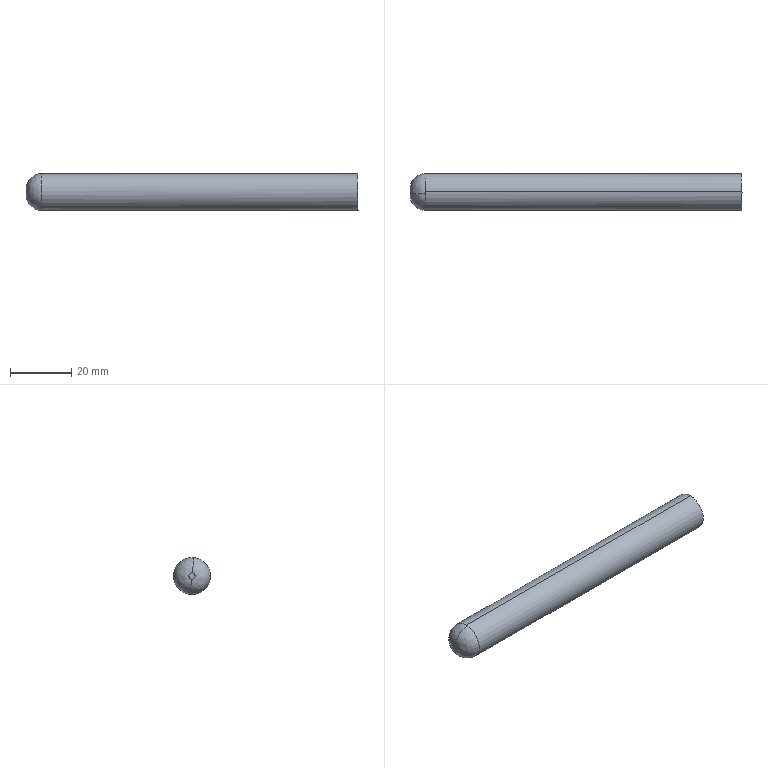Part | Creo | 1 solid | 6 faces | box 108.147 x 12 x 12 mm | volume 12066 mm3 | plane 2 | cylinder 2 | spline 2 | commonest cylinder face diameters 12 x2
STEP:
#1=CARTESIAN_POINT('',(0.,0.,0.));
#2=DIRECTION('',(0.,0.,1.));
#3=DIRECTION('',(1.,0.,0.));
#4=AXIS2_PLACEMENT_3D('',#1,#2,#3);
#5=CARTESIAN_POINT('',(-42.553,96.983,-27.835));
#6=VERTEX_POINT('',#5);
#7=CARTESIAN_POINT('',(-42.553,96.353,-39.802));
#8=VERTEX_POINT('',#7);
#9=CARTESIAN_POINT('',(-42.553,96.983,-33.835));
#10=DIRECTION('',(1.,0.,0.000000164));
#11=DIRECTION('',(-0.000000164,-0.00000002,1.));
#12=AXIS2_PLACEMENT_3D('',#9,#10,#11);
#13=CIRCLE('',#12,6.);
#14=EDGE_CURVE('',#6,#8,#13,.T.);
#15=ORIENTED_EDGE('',*,*,#14,.F.);
#16=CARTESIAN_POINT('',(-42.553,96.983,-39.835));
#17=VERTEX_POINT('',#16);
#18=CARTESIAN_POINT('',(-42.553,96.983,-33.835));
#19=DIRECTION('',(1.,0.,0.000000164));
#20=DIRECTION('',(0.000000164,0.,-1.));
#21=AXIS2_PLACEMENT_3D('',#18,#19,#20);
#22=CIRCLE('',#21,6.);
#23=EDGE_CURVE('',#17,#6,#22,.T.);
#24=ORIENTED_EDGE('',*,*,#23,.F.);
#25=CARTESIAN_POINT('',(-42.553,96.983,-33.835));
#26=DIRECTION('',(1.,0.,0.000000164));
#27=DIRECTION('',(0.000000164,-0.1051,-0.9945));
#28=AXIS2_PLACEMENT_3D('',#25,#26,#27);
#29=CIRCLE('',#28,6.);
#30=EDGE_CURVE('',#8,#17,#29,.T.);
#31=ORIENTED_EDGE('',*,*,#30,.F.);
#32=EDGE_LOOP('',(#15,#24,#31));
#33=FACE_OUTER_BOUND('',#32,.F.);
#34=CARTESIAN_POINT('',(-42.553,96.983,-33.835));
#35=DIRECTION('',(1.,0.,0.000000197));
#36=DIRECTION('',(0.000000197,0.,-1.));
#37=AXIS2_PLACEMENT_3D('',#34,#35,#36);
#38=PLANE('',#37);
#39=ADVANCED_FACE('',(#33),#38,.T.);
#40=CARTESIAN_POINT('',(-145.7,96.983,-39.835));
#41=VERTEX_POINT('',#40);
#42=CARTESIAN_POINT('',(-145.7,96.353,-27.869));
#43=VERTEX_POINT('',#42);
#44=CARTESIAN_POINT('',(-145.7,96.983,-33.835));
#45=DIRECTION('',(-1.,0.,-0.000000164));
#46=DIRECTION('',(0.000000164,0.,-1.));
#47=AXIS2_PLACEMENT_3D('',#44,#45,#46);
#48=CIRCLE('',#47,6.);
#49=EDGE_CURVE('',#41,#43,#48,.T.);
#50=ORIENTED_EDGE('',*,*,#49,.T.);
#51=CARTESIAN_POINT('',(-145.7,96.983,-27.835));
#52=VERTEX_POINT('',#51);
#53=CARTESIAN_POINT('',(-145.7,96.983,-33.835));
#54=DIRECTION('',(-1.,0.,-0.000000164));
#55=DIRECTION('',(-0.000000164,-0.1051,0.9945));
#56=AXIS2_PLACEMENT_3D('',#53,#54,#55);
#57=CIRCLE('',#56,6.);
#58=EDGE_CURVE('',#43,#52,#57,.T.);
#59=ORIENTED_EDGE('',*,*,#58,.T.);
#60=CARTESIAN_POINT('',(-42.553,96.983,-27.835));
#61=DIRECTION('',(-1.,-0.00000186,0.000000408));
#62=VECTOR('',#61,103.147);
#63=LINE('',#60,#62);
#64=EDGE_CURVE('',#6,#52,#63,.T.);
#65=ORIENTED_EDGE('',*,*,#64,.F.);
#66=ORIENTED_EDGE('',*,*,#14,.T.);
#67=ORIENTED_EDGE('',*,*,#30,.T.);
#68=CARTESIAN_POINT('',(-42.553,96.983,-39.835));
#69=DIRECTION('',(-1.,0.000001529,-0.000000164));
#70=VECTOR('',#69,103.147);
#71=LINE('',#68,#70);
#72=EDGE_CURVE('',#17,#41,#71,.T.);
#73=ORIENTED_EDGE('',*,*,#72,.T.);
#74=EDGE_LOOP('',(#50,#59,#65,#66,#67,#73));
#75=FACE_OUTER_BOUND('',#74,.F.);
#76=CARTESIAN_POINT('',(-121.87,96.983,-33.835));
#77=DIRECTION('',(-1.,0.,-0.000000164));
#78=DIRECTION('',(-0.000000164,0.,1.));
#79=AXIS2_PLACEMENT_3D('',#76,#77,#78);
#80=CYLINDRICAL_SURFACE('',#79,6.);
#81=ADVANCED_FACE('',(#75),#80,.T.);
#82=CARTESIAN_POINT('',(-145.7,97.613,-39.802));
#83=VERTEX_POINT('',#82);
#84=CARTESIAN_POINT('',(-145.7,96.983,-33.835));
#85=DIRECTION('',(-1.,0.,-0.000000164));
#86=DIRECTION('',(0.000000164,0.1051,-0.9945));
#87=AXIS2_PLACEMENT_3D('',#84,#85,#86);
#88=CIRCLE('',#87,6.);
#89=EDGE_CURVE('',#83,#41,#88,.T.);
#90=ORIENTED_EDGE('',*,*,#89,.F.);
#91=CARTESIAN_POINT('',(-150.7,97.088,-34.83));
#92=VERTEX_POINT('',#91);
#93=CARTESIAN_POINT('',(-145.7,97.088,-34.83));
#94=DIRECTION('',(0.000000017,-0.9945,-0.1051));
#95=DIRECTION('',(-1.,0.,-0.000000164));
#96=AXIS2_PLACEMENT_3D('',#93,#94,#95);
#97=CIRCLE('',#96,5.);
#98=EDGE_CURVE('',#92,#83,#97,.T.);
#99=ORIENTED_EDGE('',*,*,#98,.F.);
#100=CARTESIAN_POINT('',(-150.7,96.878,-32.841));
#101=VERTEX_POINT('',#100);
#102=CARTESIAN_POINT('',(-150.7,96.878,-32.841));
#103=CARTESIAN_POINT('',(-150.7,96.772,-32.852));
#104=CARTESIAN_POINT('',(-150.7,96.574,-32.905));
#105=CARTESIAN_POINT('',(-150.7,96.302,-33.079));
#106=CARTESIAN_POINT('',(-150.7,96.1,-33.331));
#107=CARTESIAN_POINT('',(-150.7,95.987,-33.63));
#108=CARTESIAN_POINT('',(-150.7,95.973,-33.948));
#109=CARTESIAN_POINT('',(-150.7,96.056,-34.252));
#110=CARTESIAN_POINT('',(-150.7,96.228,-34.516));
#111=CARTESIAN_POINT('',(-150.7,96.474,-34.716));
#112=CARTESIAN_POINT('',(-150.7,96.777,-34.83));
#113=CARTESIAN_POINT('',(-150.7,96.982,-34.841));
#114=CARTESIAN_POINT('',(-150.7,97.088,-34.83));
#115=B_SPLINE_CURVE_WITH_KNOTS('',3,(#102,#103,#104,#105,#106,#107,#108,#109,#110,#111,#112,#113,#114),.UNSPECIFIED.,.F.,.F.,(4,1,1,1,1,1,1,1,1,1,4),(0.,0.1,0.2,0.3,0.4,0.5,0.6,0.7,0.8,0.9,1.),.UNSPECIFIED.);
#116=EDGE_CURVE('',#101,#92,#115,.T.);
#117=ORIENTED_EDGE('',*,*,#116,.F.);
#118=CARTESIAN_POINT('',(-145.7,96.878,-32.841));
#119=DIRECTION('',(-0.000000017,0.9945,0.1051));
#120=DIRECTION('',(-1.,0.000000835,-0.00000807));
#121=AXIS2_PLACEMENT_3D('',#118,#119,#120);
#122=CIRCLE('',#121,5.);
#123=EDGE_CURVE('',#101,#43,#122,.T.);
#124=ORIENTED_EDGE('',*,*,#123,.T.);
#125=ORIENTED_EDGE('',*,*,#49,.F.);
#126=EDGE_LOOP('',(#90,#99,#117,#124,#125));
#127=FACE_OUTER_BOUND('',#126,.F.);
#128=CARTESIAN_POINT('',(-150.697,97.005,-32.994));
#129=CARTESIAN_POINT('',(-150.795,97.086,-29.919));
#130=CARTESIAN_POINT('',(-148.619,97.143,-27.743));
#131=CARTESIAN_POINT('',(-145.543,97.14,-27.84));
#132=CARTESIAN_POINT('',(-150.697,96.459,-32.979));
#133=CARTESIAN_POINT('',(-150.795,94.545,-29.852));
#134=CARTESIAN_POINT('',(-148.619,93.19,-27.639));
#135=CARTESIAN_POINT('',(-145.543,93.25,-27.738));
#136=CARTESIAN_POINT('',(-150.697,96.088,-33.381));
#137=CARTESIAN_POINT('',(-150.795,92.82,-31.719));
#138=CARTESIAN_POINT('',(-148.619,90.507,-30.544));
#139=CARTESIAN_POINT('',(-145.543,90.61,-30.596));
#140=CARTESIAN_POINT('',(-150.697,96.146,-33.924));
#141=CARTESIAN_POINT('',(-150.795,93.087,-34.247));
#142=CARTESIAN_POINT('',(-148.619,90.923,-34.476));
#143=CARTESIAN_POINT('',(-145.543,91.019,-34.466));
#144=CARTESIAN_POINT('',(-150.697,96.203,-34.467));
#145=CARTESIAN_POINT('',(-150.795,93.354,-36.775));
#146=CARTESIAN_POINT('',(-148.619,91.338,-38.408));
#147=CARTESIAN_POINT('',(-145.543,91.428,-38.335));
#148=CARTESIAN_POINT('',(-150.697,96.65,-34.782));
#149=CARTESIAN_POINT('',(-150.795,95.431,-38.24));
#150=CARTESIAN_POINT('',(-148.619,94.569,-40.687));
#151=CARTESIAN_POINT('',(-145.543,94.607,-40.578));
#152=CARTESIAN_POINT('',(-150.697,97.18,-34.654));
#153=CARTESIAN_POINT('',(-150.795,97.902,-37.644));
#154=CARTESIAN_POINT('',(-148.619,98.413,-39.76));
#155=CARTESIAN_POINT('',(-145.543,98.39,-39.666));
#156=(BOUNDED_SURFACE()B_SPLINE_SURFACE(3,3,((#128,#129,#130,#131),(#132,#133,#134,#135),(#136,#137,#138,#139),(#140,#141,#142,#143),(#144,#145,#146,#147),(#148,#149,#150,#151),(#152,#153,#154,#155)),.UNSPECIFIED.,.F.,.F.,.F.)B_SPLINE_SURFACE_WITH_KNOTS((4,3,4),(4,4),(0.,1.,2.),(0.,1.),.UNSPECIFIED.)GEOMETRIC_REPRESENTATION_ITEM()RATIONAL_B_SPLINE_SURFACE(((1.431,1.13,1.13,1.431),(1.106,0.8733,0.8733,1.106),(1.106,0.8733,0.8733,1.106),(1.431,1.13,1.13,1.431),(1.106,0.8733,0.8733,1.106),(1.106,0.8733,0.8733,1.106),(1.431,1.13,1.13,1.431)))REPRESENTATION_ITEM('')SURFACE());
#157=ADVANCED_FACE('',(#127),#156,.T.);
#158=ORIENTED_EDGE('',*,*,#89,.T.);
#159=ORIENTED_EDGE('',*,*,#72,.F.);
#160=ORIENTED_EDGE('',*,*,#23,.T.);
#161=ORIENTED_EDGE('',*,*,#64,.T.);
#162=CARTESIAN_POINT('',(-145.7,96.983,-33.835));
#163=DIRECTION('',(-1.,0.,-0.000000164));
#164=DIRECTION('',(-0.000000164,0.,1.));
#165=AXIS2_PLACEMENT_3D('',#162,#163,#164);
#166=CIRCLE('',#165,6.);
#167=EDGE_CURVE('',#52,#83,#166,.T.);
#168=ORIENTED_EDGE('',*,*,#167,.T.);
#169=EDGE_LOOP('',(#158,#159,#160,#161,#168));
#170=FACE_OUTER_BOUND('',#169,.F.);
#171=CARTESIAN_POINT('',(-121.87,96.983,-33.835));
#172=DIRECTION('',(-1.,0.,-0.000000164));
#173=DIRECTION('',(-0.000000164,0.,1.));
#174=AXIS2_PLACEMENT_3D('',#171,#172,#173);
#175=CYLINDRICAL_SURFACE('',#174,6.);
#176=ADVANCED_FACE('',(#170),#175,.T.);
#177=ORIENTED_EDGE('',*,*,#58,.F.);
#178=ORIENTED_EDGE('',*,*,#123,.F.);
#179=CARTESIAN_POINT('',(-150.7,97.088,-34.83));
#180=CARTESIAN_POINT('',(-150.7,97.194,-34.819));
#181=CARTESIAN_POINT('',(-150.7,97.393,-34.765));
#182=CARTESIAN_POINT('',(-150.7,97.664,-34.591));
#183=CARTESIAN_POINT('',(-150.7,97.866,-34.34));
#184=CARTESIAN_POINT('',(-150.7,97.979,-34.04));
#185=CARTESIAN_POINT('',(-150.7,97.993,-33.722));
#186=CARTESIAN_POINT('',(-150.7,97.909,-33.418));
#187=CARTESIAN_POINT('',(-150.7,97.739,-33.156));
#188=CARTESIAN_POINT('',(-150.7,97.493,-32.955));
#189=CARTESIAN_POINT('',(-150.7,97.188,-32.84));
#190=CARTESIAN_POINT('',(-150.7,96.984,-32.83));
#191=CARTESIAN_POINT('',(-150.7,96.878,-32.841));
#192=B_SPLINE_CURVE_WITH_KNOTS('',3,(#179,#180,#181,#182,#183,#184,#185,#186,#187,#188,#189,#190,#191),.UNSPECIFIED.,.F.,.F.,(4,1,1,1,1,1,1,1,1,1,4),(0.,0.1,0.2,0.3,0.4,0.5,0.6,0.7,0.8,0.9,1.),.UNSPECIFIED.);
#193=EDGE_CURVE('',#92,#101,#192,.T.);
#194=ORIENTED_EDGE('',*,*,#193,.F.);
#195=ORIENTED_EDGE('',*,*,#98,.T.);
#196=ORIENTED_EDGE('',*,*,#167,.F.);
#197=EDGE_LOOP('',(#177,#178,#194,#195,#196));
#198=FACE_OUTER_BOUND('',#197,.F.);
#199=CARTESIAN_POINT('',(-150.697,96.961,-34.677));
#200=CARTESIAN_POINT('',(-150.795,96.88,-37.752));
#201=CARTESIAN_POINT('',(-148.619,96.823,-39.927));
#202=CARTESIAN_POINT('',(-145.543,96.826,-39.831));
#203=CARTESIAN_POINT('',(-150.697,97.507,-34.691));
#204=CARTESIAN_POINT('',(-150.795,99.421,-37.819));
#205=CARTESIAN_POINT('',(-148.619,100.776,-40.031));
#206=CARTESIAN_POINT('',(-145.543,100.716,-39.933));
#207=CARTESIAN_POINT('',(-150.697,97.878,-34.29));
#208=CARTESIAN_POINT('',(-150.795,101.146,-35.952));
#209=CARTESIAN_POINT('',(-148.619,103.459,-37.127));
#210=CARTESIAN_POINT('',(-145.543,103.356,-37.075));
#211=CARTESIAN_POINT('',(-150.697,97.82,-33.747));
#212=CARTESIAN_POINT('',(-150.795,100.879,-33.424));
#213=CARTESIAN_POINT('',(-148.619,103.043,-33.195));
#214=CARTESIAN_POINT('',(-145.543,102.947,-33.205));
#215=CARTESIAN_POINT('',(-150.697,97.763,-33.204));
#216=CARTESIAN_POINT('',(-150.795,100.612,-30.896));
#217=CARTESIAN_POINT('',(-148.619,102.628,-29.263));
#218=CARTESIAN_POINT('',(-145.543,102.538,-29.335));
#219=CARTESIAN_POINT('',(-150.697,97.316,-32.889));
#220=CARTESIAN_POINT('',(-150.795,98.535,-29.431));
#221=CARTESIAN_POINT('',(-148.619,99.397,-26.984));
#222=CARTESIAN_POINT('',(-145.543,99.359,-27.092));
#223=CARTESIAN_POINT('',(-150.697,96.786,-33.017));
#224=CARTESIAN_POINT('',(-150.795,96.064,-30.027));
#225=CARTESIAN_POINT('',(-148.619,95.553,-27.911));
#226=CARTESIAN_POINT('',(-145.543,95.576,-28.005));
#227=(BOUNDED_SURFACE()B_SPLINE_SURFACE(3,3,((#199,#200,#201,#202),(#203,#204,#205,#206),(#207,#208,#209,#210),(#211,#212,#213,#214),(#215,#216,#217,#218),(#219,#220,#221,#222),(#223,#224,#225,#226)),.UNSPECIFIED.,.F.,.F.,.F.)B_SPLINE_SURFACE_WITH_KNOTS((4,3,4),(4,4),(0.,1.,2.),(0.,1.),.UNSPECIFIED.)GEOMETRIC_REPRESENTATION_ITEM()RATIONAL_B_SPLINE_SURFACE(((1.431,1.13,1.13,1.431),(1.106,0.8733,0.8733,1.106),(1.106,0.8733,0.8733,1.106),(1.431,1.13,1.13,1.431),(1.106,0.8733,0.8733,1.106),(1.106,0.8733,0.8733,1.106),(1.431,1.13,1.13,1.431)))REPRESENTATION_ITEM('')SURFACE());
#228=ADVANCED_FACE('',(#198),#227,.T.);
#229=ORIENTED_EDGE('',*,*,#193,.T.);
#230=ORIENTED_EDGE('',*,*,#116,.T.);
#231=EDGE_LOOP('',(#229,#230));
#232=FACE_OUTER_BOUND('',#231,.F.);
#233=CARTESIAN_POINT('',(-150.7,96.983,-33.835));
#234=DIRECTION('',(-1.,0.,-0.000000164));
#235=DIRECTION('',(-0.000000164,0.,1.));
#236=AXIS2_PLACEMENT_3D('',#233,#234,#235);
#237=PLANE('',#236);
#238=ADVANCED_FACE('',(#232),#237,.T.);
#239=CLOSED_SHELL('',(#39,#81,#157,#176,#228,#238));
#240=MANIFOLD_SOLID_BREP('',#239);
#241=(LENGTH_UNIT()NAMED_UNIT(*)SI_UNIT(.MILLI.,.METRE.));
#242=UNCERTAINTY_MEASURE_WITH_UNIT(LENGTH_MEASURE(0.01095),#241,'','');
#243=(NAMED_UNIT(*)PLANE_ANGLE_UNIT()SI_UNIT($,.RADIAN.));
#244=PLANE_ANGLE_MEASURE_WITH_UNIT(PLANE_ANGLE_MEASURE(0.01745),#243);
#245=(CONVERSION_BASED_UNIT('DEGREE',#244)NAMED_UNIT(*)PLANE_ANGLE_UNIT());
#246=(NAMED_UNIT(*)SI_UNIT($,.STERADIAN.)SOLID_ANGLE_UNIT());
#247=(GEOMETRIC_REPRESENTATION_CONTEXT(3)GLOBAL_UNCERTAINTY_ASSIGNED_CONTEXT((#242))GLOBAL_UNIT_ASSIGNED_CONTEXT((#241,#245,#246))REPRESENTATION_CONTEXT('',''));
#248=ADVANCED_BREP_SHAPE_REPRESENTATION('',(#4,#240),#247);